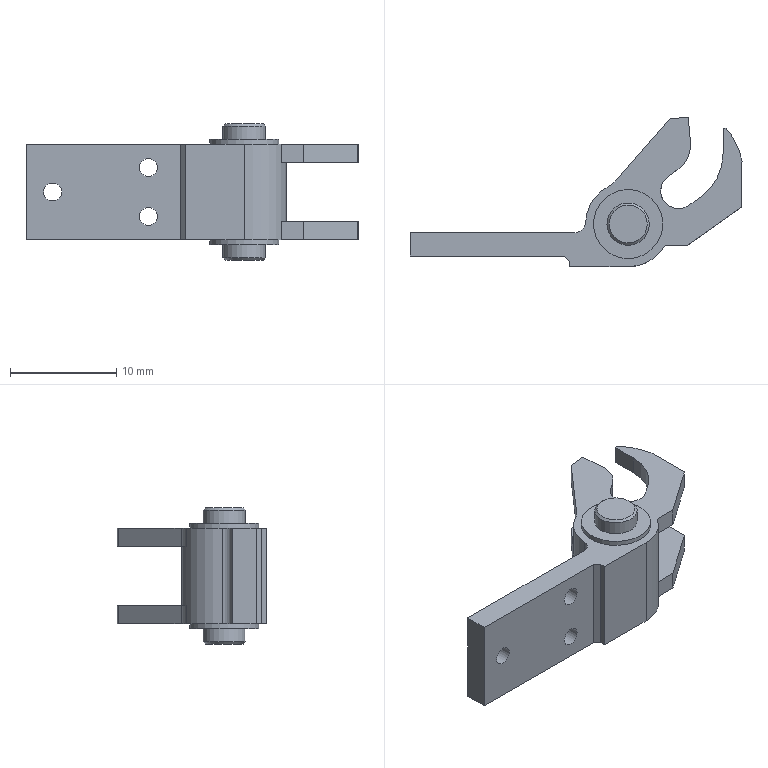NC program | NX | posted with a generic post | part box 31.196 x 14.046 x 12.8 mm
Whole program:
N10 G17 G21 G94 G90
(CAVITY_MILL , TOOL : D10-ROUGH-LOWSPEED)
N12 T00 M6
N14 G54
N16 G17 G0 G90 X-5. Y18.071 B0. C0. S4500 M3
N18 G43 Z15. H0
N20 Z2.15
N22 G94 G1 Z0.15 F800.
N24 Y13.571
N26 G3 X0. Y8.571 R5.
N28 G1 X16.073
N30 X16.6 Y8.57
N32 G2 X17.144 Y8.028 R0.545
N34 G1 X17.146 Y7.523
N36 Y-7.528
N38 X17.145 Y-8.024
N40 G2 X16.598 Y-8.57 R0.548
N42 G1 X16.073 Y-8.571
N44 X-16.073
N46 X-16.598 Y-8.57
N48 G2 X-17.145 Y-8.024 R0.548
N50 G1 X-17.146 Y-7.528
N52 Y7.523
N54 X-17.144 Y8.028
N56 G2 X-16.6 Y8.57 R0.545
N58 G1 X-16.073 Y8.571
N60 X0.
N62 Y1.071
N64 X9.646
N66 Y-1.071
N68 X-9.646
N70 Y1.071
N72 X0.
N74 G3 X5. Y6.071 R5.
N76 G1 Y18.071
N78 Z2.15
N80 G0 Z15.
N82 X-8.925 Y-18.071
N84 Z0.7
N86 G1 Z-1.3
N88 G3 X-10.302 Y-13.071 R5.
N90 G2 X-14.826 Y13.071 R22.14
N92 G1 X-5.745
N94 G3 X15.549 Y13.071 R-14.64
N96 G1 X10.095 Y7.924
N98 G2 X9.803 Y-2.17 R7.14
N100 X10.095 Y7.924 R-7.14
N102 G3 X17.163 Y7.719 R5.
N104 G1 X24.309 Y14.464
N106 Z0.7
N108 G0 Z15.
N110 X-10.964 Y-18.071
N112 Z0.25
N114 G1 Z-1.75
N116 G3 X-12.084 Y-13.071 R5.
N118 G2 X-16.231 Y13.071 R23.4
N120 G1 X-16.077
N122 X-7.42
N124 G3 X17.261 Y13.027 R-15.9
N126 G1 X11.431 Y8.308
N128 G2 X10.187 Y-3.506 R8.4
N130 X11.431 Y8.308 R-8.4
N132 G3 X18.463 Y7.567 R5.
N134 G1 X25.277 Y13.083
N136 Z0.25
N138 G0 Z15.
N140 X-26.646 Y-7.414
N142 Z-1.575
N144 G1 Z-3.575
N146 G2 X-21.646 Y-7.288 R5.
N148 G3 X-15.597 Y-8.827 R12.65
N150 G1 X-6.794
N152 G3 X-4.751 Y-10.543 R16.65
N154 G1 X-2.538 Y-13.071
N156 X3.105 Y-8.131
N158 X0.226 Y-4.842
N160 G2 X-3.148 Y-1.327 R9.15
N162 G1 X-15.595
N164 G2 X-20.748 Y3.823 R5.15
N166 G1 Y6.023
N168 G2 X-15.598 Y11.173 R5.15
N170 G1 X-3.642
N172 X-3.586 Y11.217
N174 G2 X-0.598 Y12.173 R5.15
N176 G1 X4.902
N178 G2 X10.614 Y10.171 R9.15
N180 X13.45 Y9.232 R5.15
N182 G1 X18.565 Y5.626
N184 G2 X20.748 Y1.416 R5.15
N186 G1 Y-2.877
N188 G2 X20.683 Y-3.691 R5.15
N190 X17.903 Y-9.452 R11.15
N192 X14.102 Y-11.127 R5.15
N194 G1 X13.822
N196 X13.662 Y-11.125
N198 G2 X10.099 Y-12.153 R5.15
N200 G1 X8.401 Y-12.005
N202 G2 X4.974 Y-10.267 R5.15
N204 G1 X3.105 Y-8.131
N206 G3 X-3.95 Y-7.663 R5.
N208 G1 Y-18.071
N210 Z-1.575
N212 G0 Z15.
N214 X-26.646 Y-7.414
N216 Z-3.4
N218 G1 Z-5.4
N220 G2 X-21.646 Y-7.288 R5.
N222 G3 X-15.597 Y-8.827 R12.65
N224 G1 X-6.794
N226 G3 X-4.751 Y-10.543 R16.65
N228 G1 X-2.538 Y-13.071
N230 X3.105 Y-8.131
N232 X0.226 Y-4.842
N234 G2 X-3.148 Y-1.327 R9.15
N236 G1 X-15.595
N238 G2 X-20.748 Y3.823 R5.15
N240 G1 Y6.023
N242 G2 X-15.598 Y11.173 R5.15
N244 G1 X-3.638
N246 X-3.586 Y11.217
N248 G2 X-0.598 Y12.173 R5.15
N250 G1 X4.902
N252 G2 X10.614 Y10.171 R9.15
N254 X13.45 Y9.232 R5.15
N256 G1 X18.565 Y5.626
N258 G2 X20.748 Y1.416 R5.15
N260 G1 Y-2.877
N262 G2 X20.683 Y-3.691 R5.15
N264 X17.903 Y-9.452 R11.15
N266 X14.102 Y-11.127 R5.15
N268 G1 X13.822
N270 X13.662 Y-11.125
N272 G2 X10.099 Y-12.153 R5.15
N274 G1 X8.401 Y-12.005
N276 G2 X4.974 Y-10.267 R5.15
N278 G1 X3.105 Y-8.131
N280 G3 X-3.95 Y-7.663 R5.
N282 G1 Y-18.071
N284 Z-3.4
N286 G0 Z15.
N288 X-26.646 Y-7.414
N290 Z-5.225
N292 G1 Z-7.225
N294 G2 X-21.646 Y-7.288 R5.
N296 G3 X-15.597 Y-8.827 R12.65
N298 G1 X-6.794
N300 G3 X-4.751 Y-10.543 R16.65
N302 G1 X-2.538 Y-13.071
N304 X3.105 Y-8.131
N306 X0.226 Y-4.842
N308 G2 X-3.148 Y-1.327 R9.15
N310 G1 X-15.595
N312 G2 X-20.748 Y3.823 R5.15
N314 G1 Y6.023
N316 G2 X-15.598 Y11.173 R5.15
N318 G1 X-3.638
N320 X-3.586 Y11.217
N322 G2 X-0.598 Y12.173 R5.15
N324 G1 X4.902
N326 G2 X10.614 Y10.171 R9.15
N328 X13.45 Y9.232 R5.15
N330 G1 X18.565 Y5.626
N332 G2 X20.748 Y1.416 R5.15
N334 G1 Y-2.877
N336 G2 X20.683 Y-3.691 R5.15
N338 X17.903 Y-9.452 R11.15
N340 X14.102 Y-11.127 R5.15
N342 G1 X13.822
N344 X13.662 Y-11.125
N346 G2 X10.099 Y-12.153 R5.15
N348 G1 X8.401 Y-12.005
N350 G2 X4.974 Y-10.267 R5.15
N352 G1 X3.105 Y-8.131
N354 G3 X-3.95 Y-7.663 R5.
N356 G1 Y-18.071
N358 Z-5.225
N360 G0 Z15.
N362 X-26.646 Y-7.414
N364 Z-7.05
N366 G1 Z-9.05
N368 G2 X-21.646 Y-7.288 R5.
N370 G3 X-15.597 Y-8.827 R12.65
N372 G1 X-6.794
N374 G3 X-4.751 Y-10.543 R16.65
N376 G1 X-2.538 Y-13.071
N378 X3.105 Y-8.131
N380 X0.226 Y-4.842
N382 G2 X-3.148 Y-1.327 R9.15
N384 G1 X-15.595
N386 G2 X-20.748 Y3.823 R5.15
N388 G1 Y6.023
N390 G2 X-15.598 Y11.173 R5.15
N392 G1 X-3.642
N394 X-3.586 Y11.217
N396 G2 X-0.598 Y12.173 R5.15
N398 G1 X4.902
N400 G2 X10.614 Y10.171 R9.15
N402 X13.45 Y9.232 R5.15
N404 G1 X18.565 Y5.626
N406 G2 X20.748 Y1.416 R5.15
N408 G1 Y-2.877
N410 G2 X20.683 Y-3.691 R5.15
N412 X17.903 Y-9.452 R11.15
N414 X14.102 Y-11.127 R5.15
N416 G1 X13.822
N418 X13.662 Y-11.125
N420 G2 X10.099 Y-12.153 R5.15
N422 G1 X8.401 Y-12.005
N424 G2 X4.974 Y-10.267 R5.15
N426 G1 X3.105 Y-8.131
N428 G3 X-3.95 Y-7.663 R5.
N430 G1 Y-18.071
N432 Z-7.05
N434 G0 Z15.
N436 X-26.646 Y-7.414
N438 Z-8.275
N440 G1 Z-10.275
N442 G2 X-21.646 Y-7.288 R5.
N444 G3 X-15.597 Y-8.827 R12.65
N446 G1 X-6.794
N448 G3 X-4.751 Y-10.543 R16.65
N450 G1 X-2.538 Y-13.071
N452 X3.105 Y-8.131
N454 X0.226 Y-4.842
N456 G2 X-3.148 Y-1.327 R9.15
N458 G1 X-15.595
N460 G2 X-20.748 Y3.823 R5.15
N462 G1 Y6.023
N464 G2 X-15.598 Y11.173 R5.15
N466 G1 X-3.638
N468 X-3.586 Y11.217
N470 G2 X-0.598 Y12.173 R5.15
N472 G1 X4.902
N474 G2 X10.614 Y10.171 R9.15
N476 X13.45 Y9.232 R5.15
N478 G1 X18.565 Y5.626
N480 G2 X20.748 Y1.416 R5.15
N482 G1 Y-2.877
N484 G2 X20.683 Y-3.691 R5.15
N486 X17.903 Y-9.452 R11.15
N488 X14.102 Y-11.127 R5.15
N490 G1 X13.822
N492 X13.662 Y-11.125
N494 G2 X10.099 Y-12.153 R5.15
N496 G1 X8.401 Y-12.005
N498 G2 X4.974 Y-10.267 R5.15
N500 G1 X3.105 Y-8.131
N502 G3 X-3.95 Y-7.663 R5.
N504 G1 Y-18.071
N506 Z-8.275
N508 G0 Z15.
N510 X-26.646 Y-7.414
N512 Z-9.5
N514 G1 Z-11.5
N516 G2 X-21.646 Y-7.288 R5.
N518 G3 X-15.596 Y-8.827 R12.65
N520 G1 X-6.794
N522 G3 X-4.751 Y-10.543 R16.65
N524 G1 X-2.538 Y-13.071
N526 X3.105 Y-8.131
N528 X0.226 Y-4.842
N530 G2 X-3.148 Y-1.327 R9.15
N532 G1 X-15.595
N534 G2 X-20.748 Y3.823 R5.15
N536 G1 Y6.023
N538 G2 X-15.598 Y11.173 R5.15
N540 G1 X-3.642
N542 X-3.586 Y11.218
N544 G2 X-0.598 Y12.173 R5.15
N546 G1 X4.902
N548 G2 X10.614 Y10.171 R9.15
N550 X13.45 Y9.232 R5.15
N552 G1 X18.565 Y5.626
N554 G2 X20.748 Y1.416 R5.15
N556 G1 Y-2.877
N558 G2 X20.683 Y-3.691 R5.15
N560 X17.903 Y-9.452 R11.15
N562 X14.102 Y-11.127 R5.15
N564 G1 X13.822
N566 X13.662 Y-11.125
N568 G2 X10.099 Y-12.153 R5.15
N570 G1 X8.401 Y-12.005
N572 G2 X4.974 Y-10.267 R5.15
N574 G1 X3.105 Y-8.131
N576 G3 X-3.95 Y-7.663 R5.
N578 G1 Y-18.071
N580 Z-9.5
N582 G0 Z15.
(CAVITY_MILL_COPY , TOOL : D10-ROUGH-LOWSPEED)
N584 X-14.598 Y18.171
N586 Z-4.7
N588 G1 Z-6.7 F1000.
N590 Y16.023
N592 G3 X-9.598 Y11.023 R5.
N594 G1 X-3.598
N596 G2 X-0.598 Y12.023 R5.
N598 G1 X4.902
N600 G2 X10.56 Y10.022 R9.
N602 X13.363 Y9.11 R5.
N604 G1 X18.479 Y5.503
N606 G2 X20.598 Y1.413 R5.
N608 G1 Y-2.877
N610 G2 X20.535 Y-3.667 R5.
N612 X17.792 Y-9.351 R11.
N614 X14.102 Y-10.977 R5.
N616 G1 X13.822
N618 G2 X13.614 Y-10.973 R5.
N620 X10.112 Y-12.004 R5.
N622 G1 X8.414 Y-11.855
N624 G2 X5.087 Y-10.168 R5.
N626 G1 X0.323 Y-4.725
N628 G2 X-3.058 Y-1.177 R9.
N630 G1 X-15.6
N632 G2 X-20.598 Y3.823 R5.
N634 G1 Y6.023
N636 G2 X-15.598 Y11.023 R5.
N638 G1 X-9.598
N640 G3 X-4.598 Y16.023 R5.
N642 G1 Y16.188
N644 Z-4.7
N646 G0 Z15.
N648 X-14.598 Y18.171
N650 Z-9.5
N652 G1 Z-11.5
N654 Y16.023
N656 G3 X-9.598 Y11.023 R5.
N658 G1 X-3.598
N660 G2 X-0.598 Y12.023 R5.
N662 G1 X4.902
N664 G2 X10.56 Y10.022 R9.
N666 X13.363 Y9.11 R5.
N668 G1 X18.479 Y5.503
N670 G2 X20.598 Y1.413 R5.
N672 G1 Y-2.877
N674 G2 X20.535 Y-3.667 R5.
N676 X17.792 Y-9.351 R11.
N678 X14.102 Y-10.977 R5.
N680 G1 X13.822
N682 G2 X13.614 Y-10.973 R5.
N684 X10.112 Y-12.004 R5.
N686 G1 X8.414 Y-11.855
N688 G2 X5.087 Y-10.168 R5.
N690 G1 X0.323 Y-4.725
N692 G2 X-3.058 Y-1.177 R9.
N694 G1 X-15.6
N696 G2 X-20.598 Y3.823 R5.
N698 G1 Y6.023
N700 G2 X-15.598 Y11.023 R5.
N702 G1 X-9.598
N704 G3 X-4.598 Y16.023 R5.
N706 G1 Y16.188
N708 Z-9.5
N710 G0 Z15.
(FLOOR_WALL , TOOL : D10-ROUGH-LOWSPEED)
N712 X-18.005 Y-3.177
N714 Z0.1
N716 G1 Z-1.9 F800.
N718 G3 X-17.966 Y-1.177 R5.
N720 G2 X-16.928 Y11.023 R23.25
N722 G1 X-8.665
N724 G3 X-10.278 Y-1.177 R15.75
N726 G2 X-10.141 Y-3.177 R5.
N728 G1 Z0.1
N730 G0 Z15.
N732 X7.235 Y-13.76
N734 Z0.1
N736 G1 Z-1.9
N738 G2 X9.726 Y-11.97 R5.
N740 G3 X20.598 Y1.72 R15.75
N742 G1 X13.124 Y2.341
N744 G2 X4.22 Y-5.199 R8.25
N746 X13.124 Y2.341 R-8.25
N748 G3 X17.693 Y-3.056 R5.
N750 G1 X22.598
N752 Z0.1
N754 G0 Z15.
N756 M5
(PLANAR_PROFILE , TOOL : D3-ROUGH-LOWSPEED)
N758 M6
N760 G54
N762 G17 G0 G90 X17.284 Y-9.831 B0. C0. S15000 M3
N764 G43 Z15. H0
N766 Z-0.25
N768 G94 G1 Z-2.25 F800.
N770 G41 X15.516 Y-8.063
N772 G3 X14.102 Y-7.477 R2.
N774 G1 X13.822
N776 G2 X12.322 Y-5.977 R1.5
N778 G1 Y-3.594
N780 G3 X10.839 Y-0.734 R3.5
N782 G1 X9.73 Y0.047
N784 G3 X9.486 Y0.005 R0.175
N786 X9.529 Y-0.239 R0.175
N788 G1 X10.444 Y-0.884
N790 G2 X12.25 Y-4.773 R4.3
N792 G1 X12.042 Y-7.154
N794 G3 X12.503 Y-8.614 R2.
N796 G1 X13.788 Y-10.146
N798 G40
N800 X14.109 Y-10.529
N802 Z-0.25
N804 G0 Z15.
N806 X17.284 Y-9.831
N808 Z-0.6
N810 G1 Z-2.6
N812 G41 X15.516 Y-8.063
N814 G3 X14.102 Y-7.477 R2.
N816 G1 X13.822
N818 G2 X12.322 Y-5.977 R1.5
N820 G1 Y-3.594
N822 G3 X10.839 Y-0.734 R3.5
N824 G1 X9.73 Y0.047
N826 G3 X9.486 Y0.005 R0.175
N828 X9.529 Y-0.239 R0.175
N830 G1 X10.444 Y-0.884
N832 G2 X12.25 Y-4.773 R4.3
N834 G1 X12.042 Y-7.154
N836 G3 X12.503 Y-8.614 R2.
N838 G1 X13.788 Y-10.146
N840 G40
N842 X14.109 Y-10.529
N844 Z-0.6
N846 G0 Z15.
N848 X17.284 Y-9.831
N850 Z-0.95
N852 G1 Z-2.95
N854 G41 X15.516 Y-8.063
N856 G3 X14.102 Y-7.477 R2.
N858 G1 X13.822
N860 G2 X12.322 Y-5.977 R1.5
N862 G1 Y-3.594
N864 G3 X10.839 Y-0.734 R3.5
N866 G1 X9.73 Y0.047
N868 G3 X9.486 Y0.005 R0.175
N870 X9.529 Y-0.239 R0.175
N872 G1 X10.444 Y-0.884
N874 G2 X12.25 Y-4.773 R4.3
N876 G1 X12.042 Y-7.154
N878 G3 X12.503 Y-8.614 R2.
N880 G1 X13.788 Y-10.146
N882 G40
N884 X14.109 Y-10.529
N886 Z-0.95
N888 G0 Z15.
N890 X17.284 Y-9.831
N892 Z-1.3
N894 G1 Z-3.3
N896 G41 X15.516 Y-8.063
N898 G3 X14.102 Y-7.477 R2.
N900 G1 X13.822
N902 G2 X12.322 Y-5.977 R1.5
N904 G1 Y-3.594
N906 G3 X10.839 Y-0.734 R3.5
N908 G1 X9.73 Y0.047
N910 G3 X9.486 Y0.005 R0.175
N912 X9.529 Y-0.239 R0.175
N914 G1 X10.444 Y-0.884
N916 G2 X12.25 Y-4.773 R4.3
N918 G1 X12.042 Y-7.154
N920 G3 X12.503 Y-8.614 R2.
N922 G1 X13.788 Y-10.146
N924 G40
N926 X14.109 Y-10.529
N928 Z-1.3
N930 G0 Z15.
N932 X17.284 Y-9.831
N934 Z-1.6
N936 G1 Z-3.6
N938 G41 X15.516 Y-8.063
N940 G3 X14.102 Y-7.477 R2.
N942 G1 X13.822
N944 G2 X12.322 Y-5.977 R1.5
N946 G1 Y-3.594
N948 G3 X10.839 Y-0.734 R3.5
N950 G1 X9.73 Y0.047
N952 G3 X9.486 Y0.005 R0.175
N954 X9.529 Y-0.239 R0.175
N956 G1 X10.444 Y-0.884
N958 G2 X12.25 Y-4.773 R4.3
N960 G1 X12.042 Y-7.154
N962 G3 X12.503 Y-8.614 R2.
N964 G1 X13.788 Y-10.146
N966 G40
N968 X14.109 Y-10.529
N970 Z-1.6
N972 G0 Z15.
N974 M5
N976 M2